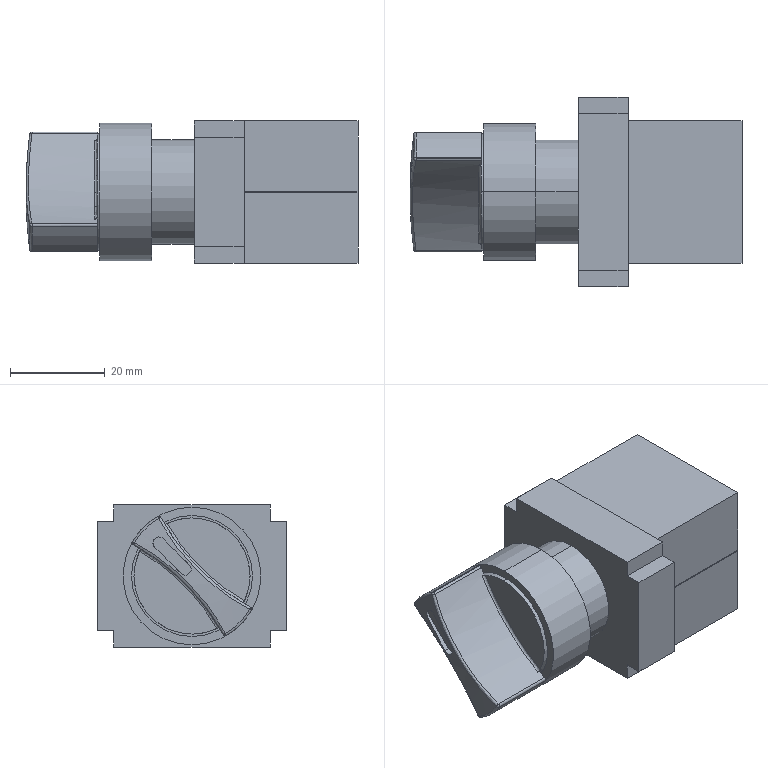Part | STEP file | Short-handle selector switch XB2-BD21C | 3 solids | 70 faces | box 70 x 40 x 30 mm | volume 44517 mm3 | plane 37 | cylinder 23 | sphere 4 | spline 4 | torus 2 | commonest cylinder face diameters 1 x5 22 x4 29 x4 2.5 x3 24.5 x2 25.5 x2